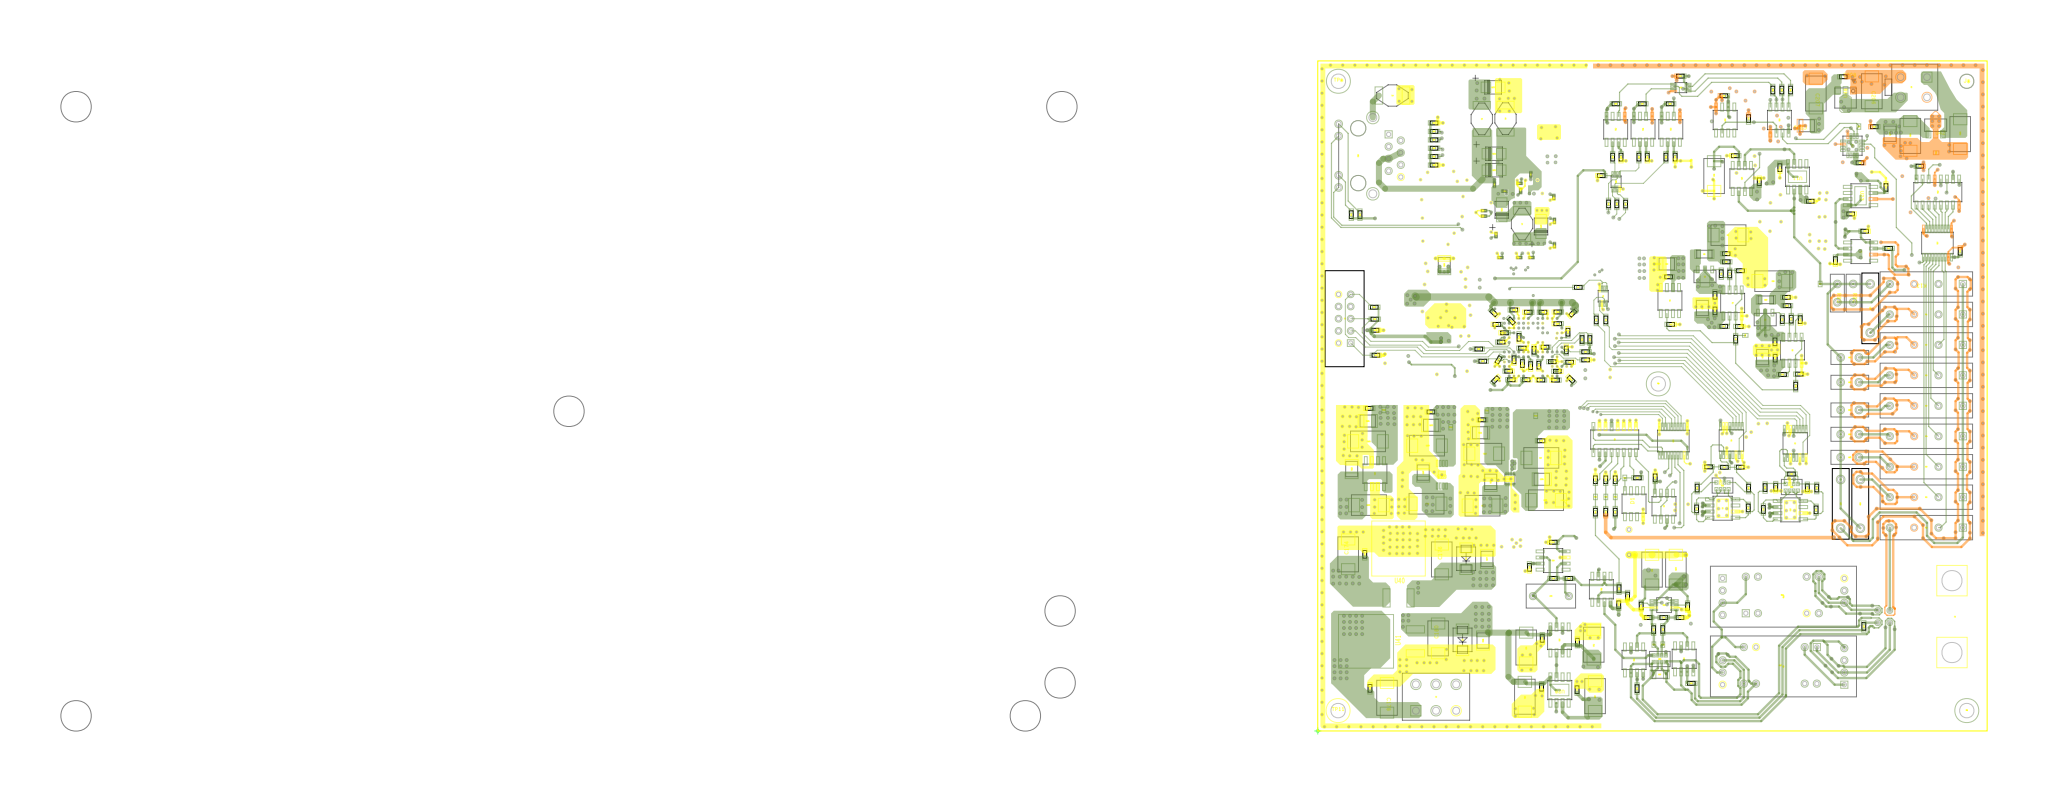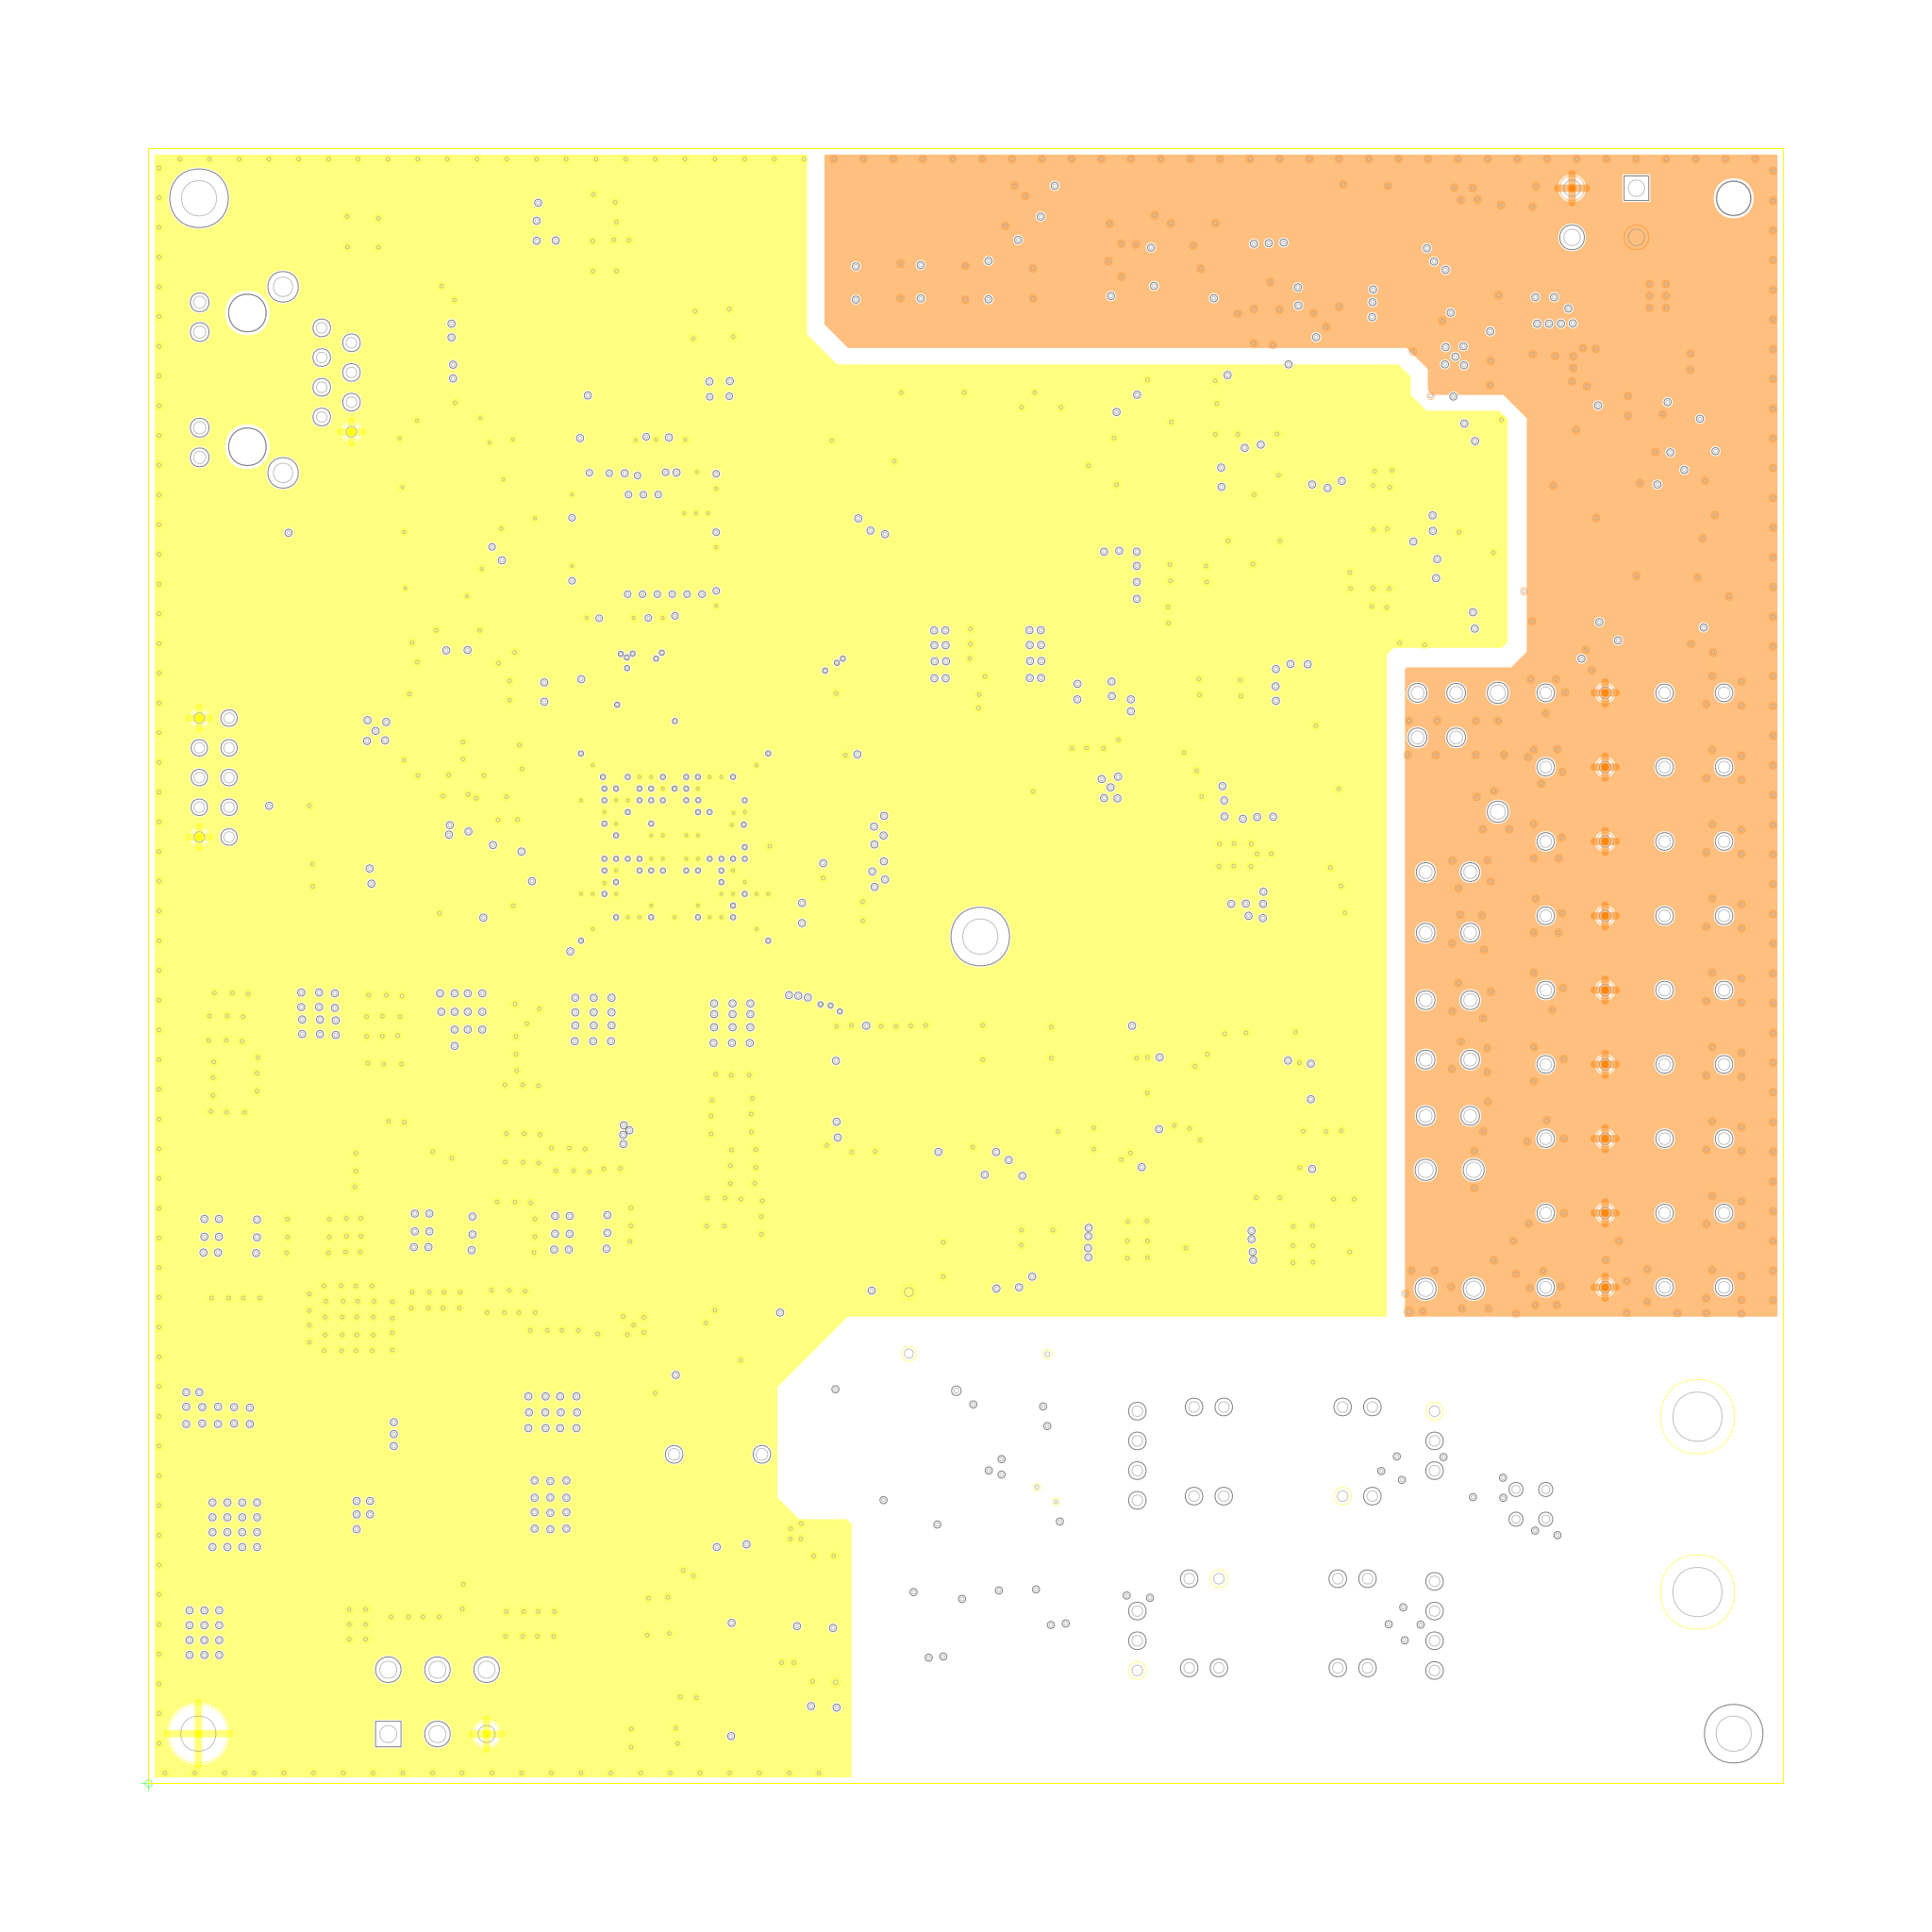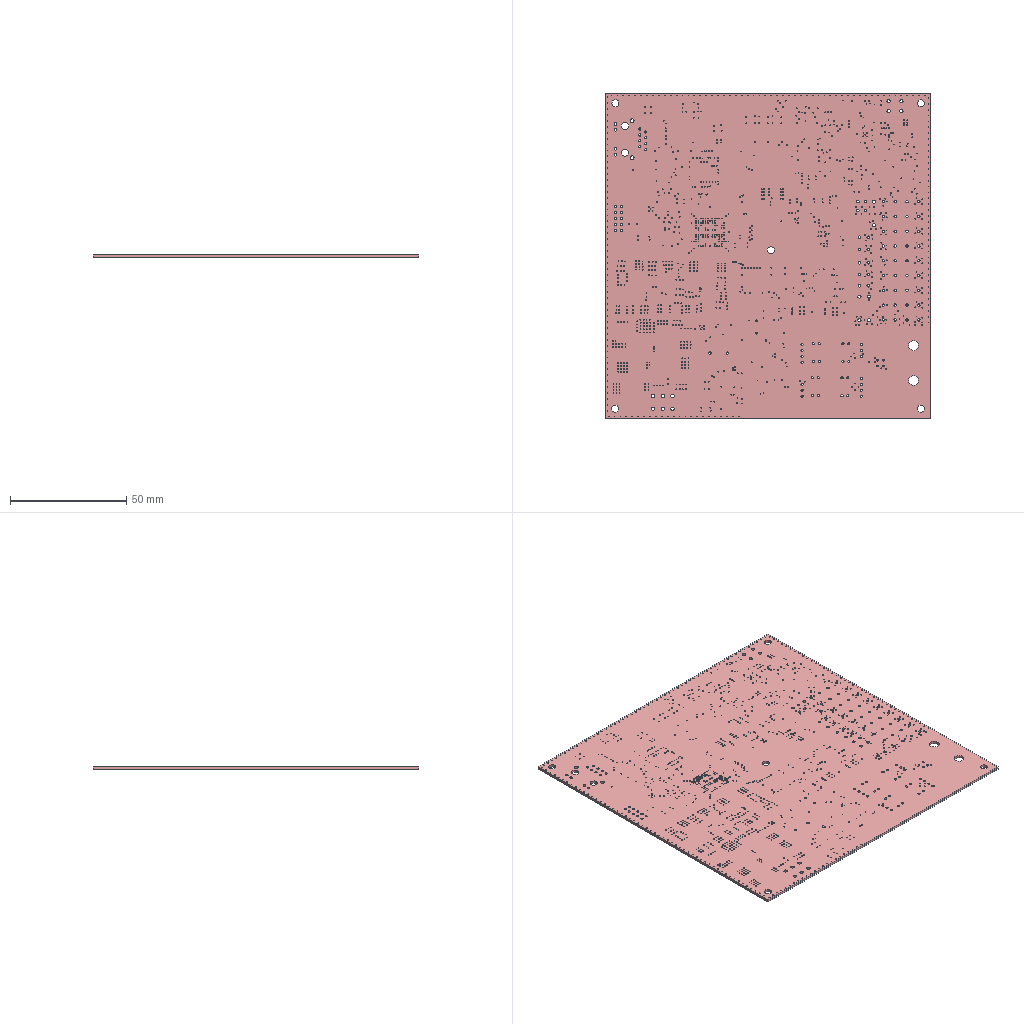Circuit board layout | Cadence Allegro | box 139.7 x 139.7 x 1.1 mm
Layer stack:
# Cadence Allegro layer stack of  (unit mm; from the constraint file cross-section; dielectric type: 0 not recorded (Allegro does not mark core vs prepreg), 3 surface material)
index,name,kind,layer,copper_thickness_mm,dielectric_type,dielectric_thickness_mm,dielectric_material,dielectric_constant
0,Top Surface,other,,,,,,
1,TOP,copper,TOP,0.0305,,,,
2,Dielectric1,dielectric,,,0,0.2032,FR-4,4.5
3,GND02,copper,GND02,0.0305,,,,
4,Dielectric2,dielectric,,,0,0.2032,FR-4,4.5
5,SIS03,copper,SIS03,0.0305,,,,
6,Dielectric3,dielectric,,,0,0.2032,FR-4,4.5
7,POW04,copper,POW04,0.0305,,,,
8,Dielectric4,dielectric,,,0,0.2032,FR-4,4.5
9,GND05,copper,GND05,0.0305,,,,
10,Dielectric5,dielectric,,,0,0.2032,FR-4,4.5
11,BOTTOM,copper,BOTTOM,0.0305,,,,
12,Bottom Surface,other,,,,,,
# drill layer pairs: low layer,high layer
drill_pair,TOP,BOTTOM
Part placement:
REFDES,COMP_VALUE,SYM_NAME,SYM_X,SYM_Y,SYM_ROTATE,SYM_MIRROR
C1,,C0603,3384.6,3751.5,270.000,NO
C2,,C0603,3263.6,3576.0,270.000,NO
C3,,C0603,3355.6,3918.0,0.000,NO
C4,,CT7343,3374.6,4070.0,0.000,NO
C5,,CT7343,3696.6,2499.0,270.000,YES
C6,,C0603,3911.6,2494.0,270.000,YES
C7,,C0603,3372.6,2403.0,0.000,YES
C8,,C0603,2882.6,3728.0,180.000,NO
C9,,C0603,3464.1,3320.0,0.000,NO
C10,,C1210,2867.6,3833.0,180.000,NO
C11,,C0603,2899.1,3337.0,0.000,NO
C12,,C1210,3160.6,3472.0,90.000,NO
C13,,C0603,3263.6,3448.0,90.000,NO
C14,,C0603,3341.6,2164.0,0.000,NO
C15,,C0603,3471.6,2165.0,0.000,NO
C16,,C0603,3210.6,2168.0,180.000,NO
C17,,C0603,3537.6,1831.0,90.000,NO
C18,,CT7343,3301.6,1695.0,180.000,YES
C19,,C0603,3039.6,1752.0,0.000,YES
C20,,C1210,3179.6,1906.0,180.000,YES
C21,,C0603,3112.6,1823.0,90.000,NO
C22,,C0603,3890.6,3380.0,270.000,NO
C23,,CT7343,3734.6,3692.0,180.000,NO
C24,,C0603,3756.6,3194.0,270.000,NO
C25,,C0603,3850.6,3559.0,0.000,NO
C26,,C0603,3561.6,2382.0,270.000,YES
C27,,CT7343,1836.6,2241.0,0.000,NO
C28,,C0603,3956.1,2929.0,0.000,NO
C29,,C1210,3654.6,3069.0,90.000,NO
C30,,C0603,3758.6,3060.0,90.000,NO
C31,,C0603,4022.6,1996.0,270.000,NO
C32,,C0603,3892.6,2109.0,0.000,NO
C33,,C0603,3762.6,2001.0,270.000,NO
C34,,C0603,2446.6,2585.0,180.000,YES
C35,,C0603,2324.6,2107.0,90.000,YES
C36,,C0603,1511.6,1447.0,270.000,YES
C37,,C0603,4094.6,1815.0,90.000,NO
C38,,CT7343,3868.6,1688.0,180.000,YES
C39,,C0603,2772.6,2078.0,90.000,NO
C40,,C0603,3604.6,1739.0,0.000,YES
C41,,C1210,3724.6,1882.0,180.000,YES
C42,,C0603,3661.6,1818.0,90.000,NO
C43,,CT7343,3256.6,4555.0,270.000,NO
C44,,C0603,4695.6,4831.0,90.000,YES
C45,,C0603,3430.6,4722.0,180.000,NO
C46,,CT7343,3966.6,4170.0,90.000,YES
C47,,C0603,4668.6,4461.0,90.000,NO
C48,,C0603,4454.6,4664.0,0.000,NO
C49,,C0603,3828.6,4902.0,0.000,YES
C50,,CT7343,3806.6,5033.0,0.000,YES
C51,,CT7343,3514.6,5126.9,270.000,YES
C52,,C0603,3539.6,5027.0,90.000,NO
C53,,C0603,3336.6,5214.0,180.000,NO
C54,,CT7343,3310.6,5125.9,270.000,YES
C55,,C0603,4322.6,4800.0,0.000,YES
C56,,C0603,4493.6,4102.0,0.000,NO
C57,,CT7343,3715.6,4302.0,270.000,YES
C58,,C0603,3627.6,4508.0,90.000,NO
C59,,CT7343,3512.6,4520.1,90.000,YES
C60,,C0603,4350.6,4698.0,90.000,YES
C61,,C0603,2462.6,4992.0,180.000,YES
C62,,C0603,4946.6,4636.0,0.000,NO
C63,,C0603,2979.6,5375.0,180.000,NO
C64,,C0603,5278.6,3937.0,90.000,NO
C65,,C0603,2672.6,4992.0,180.000,YES
C66,,CT7343,4268.6,3885.0,0.000,YES
C67,,C0603,4046.6,4348.0,0.000,NO
C68,,CT7343,4272.6,4489.0,0.000,YES
C69,,C0603,4253.6,3861.0,270.000,NO
C70,,C0603,5045.6,4330.0,0.000,YES
C71,,C0603,2903.6,4992.0,180.000,YES
C72,,CT7343,4272.6,4289.0,180.000,YES
C73,,CT7343,4273.6,4089.0,180.000,YES
C74,,C0603,3796.6,4624.0,270.000,NO
C75,,C0603,4378.6,4244.0,0.000,NO
C76,,ECQ_E1224KF,1915.6,1107.0,180.000,NO
C77,,C0603,2133.6,729.0,90.000,NO
C78,,CT7343,2267.6,707.9,90.000,NO
C79,,C0603,2130.6,339.0,90.000,NO
C80,,CT7343,2278.6,285.9,90.000,NO
C81,,C0603,1739.6,1343.0,270.000,NO
C82,,C0603,1935.6,1549.0,180.000,NO
C83,,C0603,1844.6,760.0,270.000,NO
C84,,CT7343,1712.6,684.9,90.000,NO
C85,,C0603,1838.6,359.0,270.000,NO
C86,,CT7343,1701.6,280.9,90.000,NO
C87,,C0603,2528.6,600.0,270.000,YES
C88,,C1206,2529.6,446.0,180.000,YES
C89,,C0603,2626.6,573.0,180.000,YES
C90,,C0603,2373.6,1322.0,180.000,YES
C91,,CT7343,2746.6,1324.0,90.000,NO
C92,,C0603,2714.6,931.0,0.000,NO
C93,,C0603,2657.6,1026.0,270.000,NO
C94,,C0603,2940.6,609.0,270.000,YES
C95,,C0603,2472.6,1036.0,90.000,NO
C96,,C0603,2842.6,931.0,180.000,NO
C97,,C0603,2976.6,931.0,0.000,NO
C98,,C1206,3009.6,470.0,0.000,YES
C99,,C0603,3038.6,1021.0,270.000,NO
C100,,CT7343,2942.6,1324.0,270.000,NO
C101,,C0603,3038.6,582.0,180.000,YES
C102,,C0603,2329.2,4558.5,180.000,NO
C103,,C0603,470.6,3289.0,0.000,NO
C104,,C0603,1156.6,2953.0,180.000,YES
C105,,C1210,644.6,3055.0,0.000,YES
C106,,C0603,1568.0,2953.4,0.000,NO
C107,,C0603,1485.6,3046.0,239.389,NO
C108,,C1210,1316.6,3672.0,0.000,YES
C109,,CT7343,1141.6,2322.0,90.000,YES
C110,,C0603,1534.5,3268.3,180.000,NO
C111,,C0603,1927.4,3031.3,0.000,NO
C112,,C1210,2306.6,2933.0,180.000,YES
C113,,CT7343,948.6,2318.0,90.000,YES
C114,,C0603,1610.6,3456.0,0.000,NO
C115,,C0603,1729.6,3437.0,180.000,NO
C116,,C0603,1850.6,3437.0,0.000,NO
C117,,C0603,1445.3,3432.7,315.000,NO
C118,,C0603,1972.6,3439.0,180.000,NO
C119,,C0603,2095.0,3429.2,225.000,NO
C120,,C0603,1971.6,3343.0,180.000,NO
C121,,C0603,2055.6,3273.0,90.000,NO
C122,,C0603,2081.6,2885.5,135.000,NO
C123,,C0603,1953.6,2880.0,180.000,NO
C124,,C0603,1833.6,2881.0,180.000,NO
C125,,C0603,1712.6,2883.0,0.000,NO
C126,,C0603,1589.9,2882.8,0.000,NO
C127,,C0603,1507.4,3191.9,0.000,NO
C128,,C0603,2069.4,3026.4,0.000,NO
C129,,C0603,2042.1,3127.6,90.000,NO
C130,,C0603,1145.1,3202.5,180.000,YES
C131,,C0603,1471.6,3337.0,180.000,NO
C132,,C0603,1460.0,2883.4,45.000,NO
C133,,C1210,1039.6,3824.0,90.000,NO
C134,,C0603,1103.6,3769.0,180.000,YES
C135,,C0603,970.6,3772.0,0.000,YES
C136,,C0603,1590.9,3364.8,315.000,NO
C137,,C0603,1776.6,3125.0,90.000,NO
C138,,C0603,1867.6,3150.0,180.000,NO
C139,,C0603,1748.6,2999.0,270.000,NO
C140,,C0603,1681.6,3016.0,270.000,NO
C141,,C0603,1612.6,3047.0,270.000,NO
C142,,C0603,1681.6,3142.0,0.000,NO
C143,,C0603,1968.5,2952.1,0.000,NO
C144,,C0603,1816.3,3002.6,270.000,NO
C145,,C0603,1653.6,3231.0,270.000,NO
C146,,C1210,1336.6,2585.0,0.000,YES
C147,,CT7343,1450.6,2315.0,90.000,YES
C148,,C0603,1151.6,4360.2,270.000,YES
C149,,C0603,1151.6,4242.0,90.000,YES
C150,,C0603,955.6,4991.0,180.000,NO
C151,,C3528,1448.7,4738.0,0.000,NO
C152,,C3528,1448.7,4603.0,0.000,NO
C153,,C0402,1451.6,4485.0,270.000,NO
C154,,C0603,1423.6,4639.0,270.000,YES
C155,,C3528,1834.6,4141.0,90.000,NO
C156,,C0402,1666.6,4434.0,90.000,NO
C157,,C0402,1364.6,4226.0,180.000,NO
C158,,C0402,1944.6,4186.0,270.000,NO
C159,,C0402,1754.6,3886.0,180.000,NO
C160,,C0402,1499.6,3886.0,180.000,NO
C161,,C0402,1364.6,4271.0,180.000,NO
C162,,C3528,1511.6,4278.0,90.000,NO
C163,,C0402,1750.6,4568.0,90.000,NO
C164,,C0402,1534.6,4431.0,180.000,NO
C165,,C0603,955.6,4645.0,0.000,NO
C166,,C3528,1905.6,4832.0,270.000,YES
C167,,C3528,1440.6,5283.0,0.000,NO
C168,,C0402,1656.6,4495.0,180.000,NO
C169,,C0402,1944.6,3986.0,270.000,NO
C170,,C0402,1939.6,4381.0,270.000,NO
C171,,C0402,1654.6,3886.0,180.000,NO
C172,,C0402,1464.6,4071.0,90.000,NO
C173,,C1210,4702.6,4902.0,270.000,NO
C174,,CT7343,250.0,1449.9,90.000,NO
C175,,C0603,386.0,1450.0,90.000,NO
C176,,CT7343,1019.0,1407.9,90.000,NO
C177,,C1210,1390.0,1412.0,90.000,NO
C178,,CT7343,569.0,272.1,270.000,NO
C179,,C0603,429.0,350.0,270.000,NO
C180,,CT7343,989.0,759.9,90.000,NO
C181,,C1210,1357.6,742.0,90.000,NO
C182,,CT7343,5278.6,4899.1,270.000,NO
C183,,C0603,4572.6,4960.0,180.000,NO
C184,,CT7343,4868.6,4884.1,270.000,NO
C185,,CT7343,1369.6,1507.9,270.000,YES
C186,,C0603,1882.6,1752.4,270.000,YES
C187,,CT7343,1737.6,1843.9,270.000,YES
C188,,CT7343,420.5,1854.0,0.000,NO
C189,,C1210,278.6,2150.0,90.000,NO
C190,,C0603,422.6,2648.0,180.000,NO
C191,,C1210,410.6,2544.0,180.000,NO
C192,,CT7343,412.7,2377.0,180.000,NO
C193,,C0603,1349.6,2554.0,180.000,NO
C194,,C1210,1333.6,2448.0,180.000,NO
C195,,CT7343,1367.7,2276.0,180.000,NO
C196,,CT7343,893.7,1865.0,180.000,NO
C197,,C1210,866.6,2121.0,90.000,NO
C198,,C0603,929.6,2619.0,180.000,NO
C199,,C1210,931.6,2509.0,180.000,NO
C200,,CT7343,897.7,2342.0,180.000,NO
C201,,CT7343,1353.7,1849.0,180.000,NO
C202,,C1210,1420.6,2045.0,90.000,NO
C203,,C0603,1834.6,2382.0,0.000,NO
C204,,C1210,1840.6,2066.0,0.000,NO
C205,,CT7343,1875.5,1894.0,0.000,NO
C206,,CT7343,4552.6,5251.1,270.000,NO
C207,,CT7343,4092.6,5232.1,270.000,NO
C208,,C0603,4317.6,5370.0,0.000,NO
C209,,C1210,4017.6,4968.0,180.000,NO
D1,,ASOIC_8_4MX5MX1M75_1M27,2598.7,1865.3,90.000,NO
D3,,SOT_3_1M4X3MX1M1_0M95,3838.6,689.0,180.000,YES
D5,,SOT_3_1M4X3MX1M1_0M95,3686.4,841.0,270.000,YES
D6,,SOT23,1190.1,4051.0,270.000,YES
D7,,DO-214AA,679.6,1254.0,0.000,YES
D8,,DO-214AA,1219.0,1414.0,270.000,NO
D9,,DO-214AA,1189.6,748.0,270.000,NO
D10,,DO-214AA,541.6,930.0,180.000,YES
J1,,ECG_0B_304_CLV,4650.4,938.8,180.000,NO
J2,,N2510_6002RB,220.6,3384.0,90.000,NO
J3,,39281043,5005.6,5366.7,270.000,NO
J4,,39281063,806.4,166.0,0.000,NO
K1,,COTO_9001_5_1,5000.4,3419.0,180.000,NO
K2,,COTO_9001_5_1,5000.4,1919.0,180.000,NO
K3,,COTO_9001_5_1,5000.4,2169.0,180.000,NO
K4,,COTO_9001_5_1,5000.4,2419.0,180.000,NO
K5,,COTO_9001_5_1,5000.4,2669.0,180.000,NO
K6,,COTO_9001_5_1,5000.4,2919.0,180.000,NO
K7,,COTO_9001_5_1,5000.4,3169.0,180.000,NO
K8,,COTO_9001_5_1,5000.4,1669.0,180.000,NO
K9,,COTO_3502_05_511-A,3826.4,529.8,270.000,NO
K10,,COTO_3502_05_511,3800.8,538.6,180.000,NO
K11,,COTO_3502_05_511-A,3826.4,1102.2,90.000,NO
K12,,COTO_3502_05_511,3817.1,1116.4,0.000,NO
K13,,COTO_9001_5_1,5000.4,3669.0,180.000,NO
L1,,DO1608C,1347.6,5024.0,270.000,NO
L2,,DO1608C,1678.6,4161.0,90.000,NO
L3,,DO1608C,1542.6,5026.0,270.000,NO
L4,,DO1608C,613.6,5216.0,0.000,NO
Q1,,SOT_3_2M6X4M6X1M6_1M5_C,3181.6,3788.0,180.000,NO
Q2,,SOT_3_2M6X4M6X1M6_1M5_C,3676.6,3434.0,180.000,NO
R1,,R0603,3315.6,3753.0,90.000,NO
R2,,R1206,3176.6,3914.0,0.000,NO
R3,,R0603,3356.6,3851.0,0.000,NO
R4,,R0603,3473.6,3778.0,180.000,NO
R5,,R0603,3433.6,3216.0,90.000,NO
R6,,R0603,2288.6,3374.0,90.000,NO
R7,,R0603,2140.6,3641.0,180.000,NO
R8,,R0603,3335.6,3321.0,180.000,NO
R9,,R0603,2366.6,3374.0,270.000,NO
R10,,R0603,3539.6,1994.0,90.000,NO
R11,,R0603,3117.6,1994.0,90.000,NO
R12,,R0603,3817.1,3377.0,90.000,NO
R13,,R1206,3681.6,3539.0,0.000,NO
R14,,R0603,2281.6,1796.0,90.000,NO
R15,,R0603,3855.1,3491.0,0.000,NO
R16,,R0603,2281.6,2062.0,270.000,NO
R17,,R0603,3964.6,3376.5,90.000,NO
R18,,R0603,3926.6,2831.0,90.000,NO
R19,,R0603,2365.6,1796.0,90.000,NO
R20,,R0603,2365.6,2062.0,270.000,NO
R21,,R0603,3818.6,2926.0,180.000,NO
R22,,R0603,2444.6,1796.0,90.000,NO
R23,,R0603,2444.6,2062.0,270.000,NO
R24,,R0603,4099.6,1994.0,90.000,NO
R25,,R0603,2626.6,2078.0,180.000,NO
R26,,R0603,3675.6,1998.0,90.000,NO
R27,,SM10203,4296.4,1864.0,270.000,NO
R28,,SM10203,4539.2,3469.0,270.000,NO
R29,,SM10203,4458.2,1864.0,90.000,NO
R30,,RD_2_7M87X2M91X8M53_3M81,4371.4,2246.0,0.000,NO
R31,,RD_2_7M87X2M91X8M53_3M81,4371.4,2435.0,0.000,NO
R32,,RD_2_7M87X2M91X8M53_3M81,4371.4,2635.0,0.000,NO
R33,,R0603,2449.1,5148.0,0.000,NO
R34,,R0603,2491.6,4710.0,270.000,NO
R35,,RD_2_7M87X2M91X8M53_3M81,4371.4,2862.0,0.000,NO
R36,,RD_2_7M87X2M91X8M53_3M81,4371.4,3066.0,0.000,NO
R37,,R0603,2667.1,5148.0,0.000,NO
R38,,R0603,2707.6,4710.0,270.000,NO
R39,,R0603,4690.6,3961.0,180.000,NO
R40,,R0603,2895.1,5148.0,0.000,NO
R41,,R0603,2936.6,4710.0,270.000,NO
R42,,R0603,2063.6,1252.0,0.000,NO
R43,,R0603,1936.6,1252.0,0.000,NO
R44,,R1206,2544.6,762.0,270.000,YES
R45,,R0603,2623.6,348.0,90.000,NO
R46,,R1206,2653.6,762.0,270.000,YES
R47,,R1206,2809.6,464.0,180.000,NO
R48,,R0603,2475.6,1168.0,90.000,NO
R49,,R1206,2956.6,771.0,270.000,YES
R50,,R0603,2759.6,832.0,90.000,NO
R51,,R0603,2834.6,833.0,90.000,NO
R52,,R0603,3069.6,391.0,180.000,NO
R53,,R0603,2545.6,1107.0,270.000,NO
R54,,R1206,3065.6,771.0,270.000,YES
R55,,R0603,4473.6,836.0,90.000,YES
R56,,R0603,4544.6,1110.2,0.000,YES
R57,,R0603,4486.6,858.3,270.000,NO
R58,,R0603,464.6,3478.0,0.000,NO
R59,,R0603,2171.6,3213.0,90.000,NO
R60,,R0603,1355.6,3035.0,0.000,NO
R61,,R0603,1322.6,3135.0,0.000,NO
R62,,R0603,468.6,3380.0,0.000,NO
R63,,R0603,2235.6,3213.0,90.000,NO
R64,,R0603,2200.9,3112.3,180.000,NO
R65,,R0603,477.6,3084.0,180.000,NO
R66,,R0603,2457.1,4326.4,270.000,NO
R67,,R0603,1271.6,3207.0,0.000,YES
R68,,R0603,2200.6,3046.0,0.000,NO
R69,,R0603,1148.6,3028.0,0.000,YES
R70,,R0603,2529.1,4325.0,270.000,NO
R71,,R0603,2389.1,4326.2,270.000,NO
R72,,R0603,952.6,3305.1,270.000,YES
R73,,R0603,1276.7,3295.3,0.000,YES
R74,,R0603,1223.6,4311.0,90.000,YES
R75,,R0603,1315.6,4491.0,90.000,YES
R76,,R0603,955.6,4921.0,0.000,NO
R77,,R0603,955.6,4852.0,0.000,NO
R78,,R0603,275.6,4238.0,90.000,NO
R79,,R0603,1256.6,4491.0,90.000,YES
R80,,R0603,346.6,4238.0,90.000,NO
R81,,R0603,1856.6,4627.0,90.000,YES
R82,,R0603,1921.6,4627.0,90.000,YES
R83,,R0603,1986.6,4627.0,90.000,YES
R84,,R0603,955.6,4715.0,180.000,NO
R85,,R0603,955.6,4783.0,180.000,NO
R86,,R0603,2422.6,4710.0,270.000,NO
R87,,R0603,2638.6,4710.0,270.000,NO
R88,,R0603,2860.6,4710.0,270.000,NO
R89,,R0603,3738.6,5261.0,90.000,NO
R90,,R0603,3812.6,5261.0,90.000,NO
R91,,R0603,3884.6,5261.0,90.000,NO
R92,,RD_2_7M87X2M91X8M53_3M81,4399.2,3594.0,270.000,NO
R93,,RD_2_7M87X2M91X8M53_3M81,4269.2,3594.0,270.000,NO
RN1,,ACASA,3325.6,2012.0,180.000,NO
RN2,,ACASA,3894.6,2000.0,180.000,NO
RN3,,ACASA,4275.6,4982.0,270.000,YES
RN4,,ACASA,2810.6,593.0,0.000,NO
TP1,,TP_0M8X1M15,3512.6,3247.0,270.000,NO
TP2,,TP_0M8X1M15,2281.6,1921.0,180.000,NO
TP3,,TP_0M8X1M15,2366.6,1921.0,180.000,NO
TP4,,TP_0M8X1M15,2444.6,1921.0,180.000,NO
TP5,,TP_0M8X1M15,2522.6,2077.0,180.000,NO
TP6,,TP_0M8X1M15,4445.6,4961.0,180.000,NO
TP7,,TP_0M8X1M15,4128.0,3669.0,180.000,NO
TP8,,TP_0M8X1M15,1961.6,1721.9,180.000,YES
TP9,,TP_0M8X1M15,2761.6,709.0,0.000,NO
TP10,,TP_0M8X1M15,2834.6,709.0,180.000,NO
TP11,,M3,167.2,167.2,0.000,NO
TP12,,TP_0M8X1M15,5080.6,4746.0,270.000,NO
TP13,,TP_0M8X1M15,542.6,2635.0,180.000,NO
TP14,,TP_0M8X1M15,1389.6,2630.0,180.000,NO
TP15,,TP_0M8X1M15,1092.6,2493.0,180.000,NO
TP16,,TP_0M8X1M15,1790.6,2587.0,180.000,NO
U1,,SOIC_8_4MX5MX1M75_1M27,3408.6,3513.0,90.000,NO
U2,,SOIC_8_4MX5MX1M75_1M27,2893.6,3533.0,270.000,NO
U3,,SOPTS_16_4M5X5M1X1M2_0M65,3398.6,2384.0,90.000,NO
U4,,SOPVS_8_2M4X2M1X0M9_0M5,2345.6,3569.0,270.000,NO
U5,,SOIC8,3326.6,1828.0,270.000,NO
U6,,SOIC_8_4MX5MX1M75_1M27,3900.6,3125.0,90.000,NO
U7,,SOPTS_16_4M5X5M1X1M2_0M65,3923.0,2360.9,90.000,NO
U8,,SOIC_16_4MX10MX1M75_1M27,2439.6,2392.0,90.000,NO
U9,,SOIC_8_4MX5MX1M75_1M27,2844.6,1845.0,270.000,NO
U10,,SOIC8,3883.6,1815.0,270.000,NO
U11,,TO220_5_10M67X4M83X16M11_1M7_B,3941.7,4549.0,180.000,NO
U12,,QFN_17_4MX4MX1M_0M65,4393.6,4804.0,270.000,NO
U13,,SOIC_8_4MX5MX1M75_1M27,3484.6,4535.0,90.000,NO
U14,,SOIC_8_4MX5MX1M75_1M27,4540.6,4839.0,270.000,YES
U15,,SOIC_8_4MX5MX1M75_1M27,3793.6,5015.0,270.000,NO
U16,,SOIC_8_4MX5MX1M75_1M27,3347.6,5015.0,270.000,NO
U17,,SOPTS_20_4M5X6M6X1M2_0M65,5091.6,4005.0,270.000,NO
U18,,SOIC_8_4MX5MX1M75_1M27,2447.6,4938.0,90.000,NO
U19,,SOIC_16_4MX10MX1M75_1M27,5094.6,4423.0,90.000,NO
U20,,SOPVS_8_2M4X2M1X0M9_0M5,2983.6,5281.0,0.000,NO
U21,,SOIC_8_4MX5MX1M75_1M27,2672.6,4939.0,90.000,NO
U22,,SOIC_8_4MX5MX1M75_1M27,4460.3,3935.0,180.000,NO
U23,,TO220_5_10M67X4M83X16M11_1M7_B,4459.6,4393.1,270.000,NO
U24,,SOIC_16_4MX10MX1M75_1M27,5046.6,4082.0,180.000,YES
U25,,SOIC_8_4MX5MX1M75_1M27,2900.6,4939.0,90.000,NO
U26,,SOIC_8_4MX5MX1M75_1M27,1933.6,1399.0,180.000,NO
U27,,SOIC_8_4MX5MX1M75_1M27,1986.5,747.0,270.000,NO
U28,,TO220_5_10M67X4M83X16M11_1M7_B,1988.6,336.0,180.000,NO
U29,,SOIC_8_4MX5MX1M75_1M27,2598.6,583.0,90.000,NO
U30,,SOPTS_20_4M5X6M6X1M2_0M65,2921.6,2380.0,270.000,NO
U31,,SOIC_8_4MX5MX1M75_1M27,2330.6,1163.0,90.000,NO
U32,,SOPM_10_3M1X3M1X1M1_0M5,2845.6,1033.0,180.000,NO
U33,,BGA_256_17MX17MX1M55_1M,1769.6,3150.0,180.000,YES
U34,,SOIC_8_4MX5MX1M75_1M27,924.8,3002.2,0.000,YES
U35,,SOPVS_8_2M4X2M1X0M9_0M5,1091.6,3304.1,180.000,YES
U36,,SOPVS_8_2M4X2M1X0M9_0M5,2451.3,4507.7,90.000,NO
U37,,CO4-5R0X7R0-S,1041.6,3576.0,90.000,YES
U38,,100-LQFP,1667.9,4159.4,90.000,YES
U39,,RJ45,332.4,4722.0,90.000,NO
U40,,TO-263-2,663.5,1497.5,0.000,NO
U41,,TO-263-2,396.5,735.5,90.000,NO
U42,,UA78L05ACPK_SOT_3,5077.0,4895.4,0.000,NO
U43,,SOIC_8_4MX5MX1M75_1M27,469.6,2112.0,270.000,NO
U44,,UA78L05ACPK_SOT_3,1741.2,1541.0,90.000,YES
U45,,MINI_SO_EP_8,1019.6,2103.0,180.000,NO
U46,,DFN_9_2M1X2M1X0M6_0M5,1578.6,2068.0,90.000,NO
U47,,SOIC_8_4MX5MX1M75_1M27,3010.6,592.0,90.000,NO
U48,,L79L05ABUTR,4336.4,5258.4,90.000,NO
U49,,TO220_5_10M67X4M83X16M11_1M7_B,3961.0,4630.0,180.000,YES
U50,,TO220_5_10M67X4M83X16M11_1M7_B,4703.0,4150.9,270.000,YES
U51,,TO220_5_10M67X4M83X16M11_1M7_B,2038.0,671.0,270.000,YES
Y1,,CO2-4R8X11R1-S,991.6,4299.0,270.000,YES
Pad and via stacks:
# Allegro (Cadence) via spans and padstacks; design units: ("mils" 1 10)
# via spans: padstack,start_layer,end_layer,net_example,count
VIA0M45X0M25,ETCH/TOP,ETCH/BOTTOM,GND,113
VIA10-F,ETCH/BOTTOM,ETCH/TOP,GND,48
V50D30,ETCH/TOP,ETCH/BOTTOM,GND,2
VIA10-F,ETCH/TOP,ETCH/BOTTOM,LINKLED,4
VIA24X12,ETCH/TOP,ETCH/BOTTOM,GND,1166
V32D16,ETCH/TOP,ETCH/BOTTOM,GND,4
# Allegro padstack definitions: name,start_layer,end_layer,drill,plating,holeType,type
SMD1R60X2R70,"ETCH/TOP","ETCH/TOP",0.0,"PLATED","none","smd"
SMD0R76X0R80,"ETCH/TOP","ETCH/TOP",0.0,"PLATED","none","smd"
SMD1R20X1R60,"ETCH/TOP","ETCH/TOP",0.0,"PLATED","none","smd"
SMD2R00X2R20,"ETCH/TOP","ETCH/TOP",0.0,"PLATED","none","smd"
SMD0R51X0R51,"ETCH/TOP","ETCH/TOP",0.0,"PLATED","none","smd"
SMD1R00X1R40,"ETCH/TOP","ETCH/TOP",0.0,"PLATED","none","smd"
SMD1R60X3R60,"ETCH/TOP","ETCH/TOP",0.0,"NON_PLATED","none","smd"
SMD1R00X1R00,"ETCH/TOP","ETCH/TOP",0.0,"PLATED","none","smd"
SMD65REC13,"ETCH/TOP","ETCH/TOP",0.0,"PLATED","none","smd"
SMD1R80X2R00,"ETCH/TOP","ETCH/TOP",0.0,"PLATED","none","smd"
SMDF0R28X1R80,"ETCH/TOP","ETCH/TOP",0.0,"PLATED","none","smd"
SMDF1R80X0R28,"ETCH/TOP","ETCH/TOP",0.0,"NON_PLATED","none","smd"
SMDF1R00X0R40,"ETCH/TOP","ETCH/TOP",0.0,"PLATED","none","smd"
SMD3R10X3R10,"ETCH/TOP","ETCH/TOP",0.0,"PLATED","none","smd"
SMD1R50X5R00,"ETCH/TOP","ETCH/TOP",0.0,"PLATED","none","smd"
R640_285,"ETCH/TOP","ETCH/TOP",0.0,"NON_PLATED","none","smd"
SMD1R15X0R80,"ETCH/TOP","ETCH/TOP",0.0,"PLATED","none","smd"
R1M70X0M60,"ETCH/TOP","ETCH/TOP",0.0,"PLATED","none","smd"
R198-12_55-88,"ETCH/TOP","ETCH/TOP",0.0,"NON_PLATED","none","smd"
R142-5_45,"ETCH/TOP","ETCH/TOP",0.0,"NON_PLATED","none","smd"
R294-7_175-3,"ETCH/TOP","ETCH/TOP",0.0,"NON_PLATED","none","smd"
R2M70X1M20,"ETCH/TOP","ETCH/TOP",0.0,"PLATED","none","smd"
R0M90X0M85,"ETCH/TOP","ETCH/TOP",0.0,"PLATED","none","smd"
R2M80X2M30,"ETCH/TOP","ETCH/TOP",0.0,"PLATED","none","smd"
R1M80X1M20,"ETCH/TOP","ETCH/TOP",0.0,"PLATED","none","smd"
SMD20_17,"ETCH/TOP","ETCH/TOP",0.0,"PLATED","none","smd"
R1M20X0M90,"ETCH/TOP","ETCH/TOP",0.0,"PLATED","none","smd"
R1M40X0M60,"ETCH/TOP","ETCH/TOP",0.0,"PLATED","none","smd"
SOT89_3_PIN,"ETCH/TOP","ETCH/TOP",0.0,"PLATED","none","smd"
R0M70X0M64,"ETCH/TOP","ETCH/TOP",0.0,"PLATED","none","smd"
R0M70X0M50,"ETCH/TOP","ETCH/TOP",0.0,"PLATED","none","smd"
R1M60X0M40,"ETCH/TOP","ETCH/TOP",0.0,"PLATED","none","smd"
R1M25X0M30,"ETCH/TOP","ETCH/TOP",0.0,"PLATED","none","smd"
R2M25X1M85,"ETCH/TOP","ETCH/TOP",0.0,"PLATED","none","smd"
R1M10X0M40,"ETCH/TOP","ETCH/TOP",0.0,"PLATED","none","smd"
S2M35,"ETCH/TOP","ETCH/TOP",0.0,"PLATED","none","smd"
R1M00X0M40,"ETCH/TOP","ETCH/TOP",0.0,"PLATED","none","smd"
R1M60X0M30,"ETCH/TOP","ETCH/TOP",0.0,"PLATED","none","smd"
C0M50,"ETCH/TOP","ETCH/TOP",0.0,"PLATED","none","smd"
R2M40X1M65,"ETCH/TOP","ETCH/TOP",0.0,"PLATED","none","smd"
R0M70X0M25,"ETCH/TOP","ETCH/TOP",0.0,"PLATED","none","smd"
R1M50X1M00,"ETCH/TOP","ETCH/TOP",0.0,"PLATED","none","smd"
UA78L05ACPK_PIN2,"ETCH/TOP","ETCH/TOP",0.0,"PLATED","none","smd"
R105_55,"ETCH/TOP","ETCH/TOP",0.0,"NON_PLATED","none","smd"
R1M70X1M10,"ETCH/TOP","ETCH/TOP",0.0,"PLATED","none","smd"
R0M60X0M25,"ETCH/TOP","ETCH/TOP",0.0,"PLATED","none","smd"
R1M70X0M80,"ETCH/TOP","ETCH/TOP",0.0,"PLATED","none","smd"
THC2R60D1R65,"ETCH/TOP","ETCH/BOTTOM",65.0,"PLATED","circle_drill","through"
THC1R60D1R05,"ETCH/TOP","ETCH/BOTTOM",41.3,"PLATED","circle_drill","through"
THC0R00D3R20,"ETCH/TOP","ETCH/BOTTOM",126.0,"NON_PLATED","circle_drill","through"
THC1R50D0R90,"ETCH/TOP","ETCH/BOTTOM",35.4,"PLATED","circle_drill","through"
THS1R50D0R90,"ETCH/TOP","ETCH/BOTTOM",35.4,"PLATED","circle_drill","through"
CD1M30X0M90,"ETCH/TOP","ETCH/BOTTOM",35.4,"PLATED","circle_drill","through"
CD1M50X1M00,"ETCH/TOP","ETCH/BOTTOM",39.4,"PLATED","circle_drill","through"
CD50X28,"ETCH/TOP","ETCH/BOTTOM",28.7,"PLATED","circle_drill","through"
C123_H73,"ETCH/TOP","ETCH/BOTTOM",28.7,"PLATED","circle_drill","through"
CD1M40X0M90,"ETCH/TOP","ETCH/BOTTOM",35.4,"PLATED","circle_drill","through"
SD1M40X0M90,"ETCH/TOP","ETCH/BOTTOM",35.4,"PLATED","circle_drill","through"
CD1M20X0M70,"ETCH/TOP","ETCH/BOTTOM",27.6,"PLATED","circle_drill","through"
SD6M35X4M20,"ETCH/TOP","ETCH/BOTTOM",165.4,"PLATED","circle_drill","through"
S217-5_H145,"ETCH/TOP","ETCH/BOTTOM",57.1,"PLATED","circle_drill","through"
C217-5_H145,"ETCH/TOP","ETCH/BOTTOM",57.1,"PLATED","circle_drill","through"
SD1M50X1M00,"ETCH/TOP","ETCH/BOTTOM",39.4,"PLATED","circle_drill","through"
CD1M50X0M90,"ETCH/TOP","ETCH/BOTTOM",35.4,"PLATED","circle_drill","through"
SD1M50X0M90,"ETCH/TOP","ETCH/BOTTOM",35.4,"PLATED","circle_drill","through"
CD1M80X1M30,"ETCH/TOP","ETCH/BOTTOM",51.2,"PLATED","circle_drill","through"
CD1M60X1M10,"ETCH/TOP","ETCH/BOTTOM",43.3,"PLATED","circle_drill","through"
SD6M35X4M20_NP,"ETCH/TOP","ETCH/BOTTOM",165.4,"NON_PLATED","circle_drill","through"
SD1M80X1M30,"ETCH/TOP","ETCH/BOTTOM",51.2,"PLATED","circle_drill","through"
S210_H140,"ETCH/TOP","ETCH/BOTTOM",55.1,"PLATED","circle_drill","through"
C210_H140,"ETCH/TOP","ETCH/BOTTOM",55.1,"PLATED","circle_drill","through"
VIA24X12,"ETCH/TOP","ETCH/BOTTOM",12.0,"PLATED","circle_drill","through"
VIA0M45X0M25,"ETCH/TOP","ETCH/BOTTOM",9.8,"PLATED","circle_drill","through"
VIA,"ETCH/TOP","ETCH/BOTTOM",13.0,"PLATED","circle_drill","through"
VIA10-F,"ETCH/TOP","ETCH/BOTTOM",9.8,"PLATED","circle_drill","through"
VIA24X12_S,"ETCH/TOP","ETCH/BOTTOM",12.0,"PLATED","circle_drill","through"
R0M90X0M85-1,"ETCH/TOP","ETCH/TOP",0.0,"PLATED","none","smd"
PAD156,"ETCH/TOP","ETCH/BOTTOM",156.0,"NON_PLATED","circle_drill","through"
HOLE109P,"ETCH/TOP","ETCH/BOTTOM",108.0,"PLATED","circle_drill","through"
PAD125,"ETCH/TOP","ETCH/BOTTOM",126.0,"NON_PLATED","circle_drill","through"
SMD2M61_2M02,"ETCH/TOP","ETCH/TOP",0.0,"PLATED","none","smd"
SMD71_25,"ETCH/TOP","ETCH/TOP",0.0,"PLATED","none","smd"
SMD3M80_2M40,"ETCH/TOP","ETCH/TOP",0.0,"PLATED","none","smd"
A_SOT89,"ETCH/TOP","ETCH/TOP",0.0,"NON_PLATED","none","smd"
R45X60,"ETCH/TOP","ETCH/TOP",0.0,"NON_PLATED","none","smd"
SMD3M00_1M60,"ETCH/TOP","ETCH/TOP",0.0,"PLATED","none","smd"
SMD6M20_5M80,"ETCH/TOP","ETCH/TOP",0.0,"PLATED","none","smd"
SMD0M35_1M30,"ETCH/TOP","ETCH/TOP",0.0,"PLATED","none","smd"
PAD5M00CIR2M03D,"ETCH/TOP","ETCH/BOTTOM",118.1,"PLATED","circle_drill","through"
V32D16,"ETCH/TOP","ETCH/BOTTOM",16.0,"PLATED","circle_drill","through"
V50D30,"ETCH/TOP","ETCH/BOTTOM",30.0,"PLATED","circle_drill","through"
R1_52X3_81,"ETCH/TOP","ETCH/TOP",0.0,"PLATED","none","smd"
R11_18X11_48-NSP,"ETCH/TOP","ETCH/TOP",0.0,"PLATED","none","smd"
R1_5X1_6,"ETCH/TOP","ETCH/TOP",0.0,"NON_PLATED","none","smd"
HOLE1P9,"ETCH/TOP","ETCH/BOTTOM",74.8,"NON_PLATED","circle_drill","through"
H0300,"ETCH/TOP","ETCH/BOTTOM",118.1,"NON_PLATED","circle_drill","through"
Design rules, without the lines most boards share, first 11 of 48 lines:
# Cadence Allegro design rules of  (from the Constraint Manager export constraints.dcfx, design unit mil; typed fields in mm)
# columns: name | kind | enabled | priority | scope1 | scope2 | descriptor | typed fields (field=value)
# Allegro precedence (priority 1 wins): 1 Region class-to-class, 2 Region class, 3 Region, 4 class-to-class, 5 DiffPair/Bus/NetGroup override, 6 NetClass, 7 constraint set (CSet) default
# per-layer values are written LAYER=value in the descriptor and LAYER:mm in the typed field; a maximum of 0 means no limit set
# --- net classes (and buses / net groups) ---
# (no net classes defined: every net uses the default constraint sets)
# --- track widths, neck and differential-pair gap (physical constraint sets) ---
DEFAULT | PhysicalCSet | enabled | 7 | Design default | All | Physical Constraint (Min Line Width=6mil) (Max Line Width=0mil) (Min Neck Width=6mil) (Max Neck Length=0mil) (DiffPair Primary Gap=0mil) (DiffPair Neck Gap=0mil) (DiffPair Min Space=0mil) (DiffPair Coupled +Tol=0mil) (DiffPair Coupled -Tol=0mil) (Min BB Via Stagger=5mil) (Max BB Via Stagger=0mil) (T-junctions=ANYWHERE) (Pad-pad direct connect=ALL_ALLOWED) (Allowed vias=VIA24X12, VIA0M45X0M25, VIA10-F) | min_line_width=0.1524 min_neck_width=0.1524 min_bvia_stagger=0.127 max_bvia_stagger=0 ts_allowed=ANYWHERE diffp_primary_gap=0 diffp_neck_gap=0 max_line_width=0 maximum_neck_length=0 pad_pad_direct_connect=ALL_ALLOWED allow_on_etch_subclass=TRUE diffp_coupled_plus=0 diffp_coupled_minus=0 diffp_min_space=0 vias=VIA24X12,VIA0M45X0M25,VIA10-F
# --- clearances: line / pad / via / shape / hole (spacing constraint sets) ---
HAP | SpacingCSet | enabled | 7 | Region(1): 10 | All | Clearance Constraint (Line-Line=8mil) (Line-SMD Pad=6mil) (Line-Thru Pin=6mil) (Line-Via=7mil) (Line-Shape=TOP=10mil GND02=10mil SIS03=10mil POW04=20mil GND05=20mil BOTTOM=10mil) (SMD Pad-SMD Pad=5mil) (Thru Pin-Thru Pin=5mil) (Thru Pin-SMD Pad=5mil) (SMD Pad-Via=5mil) (Thru Pin-Via=5mil) (Via-Via=5mil) (Shape-SMD Pad=5mil) (Shape-Thru Pin=5mil) (Shape-Via=5mil) (Shape-Shape=TOP=10mil GND02=40mil SIS03=20mil POW04=20mil GND05=20mil BOTTOM=10mil) (Hole-Hole=8mil) (Hole-Line=8mil) (Hole-Shape=8mil) (BB Via-BB Via=5mil) (uVia-uVia=5mil) | thrupin_to_thrupin_spacing=0.127 thrupin_to_smdpin_spacing=0.127 thrupin_to_thruvia_spacing=0.127 line_to_thrupin_spacing=0.1524 thrupin_to_shape_spacing=0.127 smdpin_to_smdpin_spacing=0.127 smdpin_to_thruvia_spacing=0.127 line_to_smdpin_spacing=0.1524 shape_to_smdpin_spacing=0.127 thruvia_to_thruvia_spacing=0.127 line_to_thruvia_spacing=0.1778 shape_to_thruvia_spacing=0.127 line_to_line_spacing=0.2032 line_to_shape_spacing=TOP:0.254,GND02:0.254,SIS03:0.254,POW04:0.508,GND05:0.508,BOTTOM:0.254 shape_to_shape_spacing=TOP:0.254,GND02:1.016,SIS03:0.508,POW04:0.508,GND05:0.508,BOTTOM:0.254 bbv_to_bbv_spacing=0.127 bbv_to_thrupin_spacing=0.127 bbv_to_smdpin_spacing=0.127 bbv_to_thruvia_spacing=0.127 bbv_to_line_spacing=0.1778 bbv_to_shape_spacing=0.127 bbv_to_testpin_spacing=0.127 bbv_to_testvia_spacing=0.127 testpin_to_testpin_spacing=0.127 testpin_to_thrupin_spacing=0.127 smdpin_to_testpin_spacing=0.127 testpin_to_thruvia_spacing=0.127 testpin_to_testvia_spacing=0.127 line_to_testpin_spacing=0.1524 shape_to_testpin_spacing=0.127 testvia_to_testvia_spacing=0.127 testvia_to_thrupin_spacing=0.127 smdpin_to_testvia_spacing=0.127 testvia_to_thruvia_spacing=0.127 line_to_testvia_spacing=0.1778 shape_to_testvia_spacing=0.127 bondpad_to_bondpad_spacing=0.127 thrupin_to_bondpad_spacing=0.127 smdpin_to_bondpad_spacing=0.127 bondpad_to_thruvia_spacing=0.127 bondpad_to_line_spacing=0.1778 bondpad_to_shape_spacing=0.127 bondpad_to_bbv_spacing=0.127 bondpad_to_testpin_spacing=0.127 bondpad_to_testvia_spacing=0.127 min_bvia_gap=0.127 hole_to_pin_spacing=0.2032 hole_to_via_spacing=0.2032 hole_to_line_spacing=0.2032 hole_to_shape_spacing=0.2032 hole_to_hole_spacing=0.2032 mvia_to_mvia_spacing=0.127 mvia_to_thrupin_spacing=0.127 mvia_to_smdpin_spacing=0.127 mvia_to_thruvia_spacing=0.127 mvia_to_bbv_spacing=0.127 mvia_to_line_spacing=0.127 mvia_to_shape_spacing=0.127 mvia_to_testpin_spacing=0.127 mvia_to_testvia_spacing=0.127 bondpad_to_mvia_spacing=0.127 bondpad_to_bondpad_diffp_spc=0.127
DEFAULT | SpacingCSet | enabled | 7 | Design default | All | Clearance Constraint (Line-Line=8mil) (Line-SMD Pad=6mil) (Line-Thru Pin=6mil) (Line-Via=7mil) (Line-Shape=TOP=10mil GND02=10mil SIS03=10mil POW04=20mil GND05=20mil BOTTOM=10mil) (SMD Pad-SMD Pad=5mil) (Thru Pin-Thru Pin=5mil) (Thru Pin-SMD Pad=5mil) (SMD Pad-Via=5mil) (Thru Pin-Via=5mil) (Via-Via=5mil) (Shape-SMD Pad=5mil) (Shape-Thru Pin=5mil) (Shape-Via=5mil) (Shape-Shape=TOP=20mil GND02=40mil SIS03=20mil POW04=20mil GND05=20mil BOTTOM=20mil) (Hole-Hole=8mil) (Hole-Line=8mil) (Hole-Shape=8mil) (BB Via-BB Via=5mil) (uVia-uVia=5mil) | thrupin_to_thrupin_spacing=0.127 thrupin_to_smdpin_spacing=0.127 thrupin_to_thruvia_spacing=0.127 line_to_thrupin_spacing=0.1524 thrupin_to_shape_spacing=0.127 smdpin_to_smdpin_spacing=0.127 smdpin_to_thruvia_spacing=0.127 line_to_smdpin_spacing=0.1524 shape_to_smdpin_spacing=0.127 thruvia_to_thruvia_spacing=0.127 line_to_thruvia_spacing=0.1778 shape_to_thruvia_spacing=0.127 line_to_line_spacing=0.2032 line_to_shape_spacing=TOP:0.254,GND02:0.254,SIS03:0.254,POW04:0.508,GND05:0.508,BOTTOM:0.254 shape_to_shape_spacing=TOP:0.508,GND02:1.016,SIS03:0.508,POW04:0.508,GND05:0.508,BOTTOM:0.508 bbv_to_bbv_spacing=0.127 bbv_to_thrupin_spacing=0.127 bbv_to_smdpin_spacing=0.127 bbv_to_thruvia_spacing=0.127 bbv_to_line_spacing=0.1778 bbv_to_shape_spacing=0.127 bbv_to_testpin_spacing=0.127 bbv_to_testvia_spacing=0.127 testpin_to_testpin_spacing=0.127 testpin_to_thrupin_spacing=0.127 smdpin_to_testpin_spacing=0.127 testpin_to_thruvia_spacing=0.127 testpin_to_testvia_spacing=0.127 line_to_testpin_spacing=0.1524 shape_to_testpin_spacing=0.127 testvia_to_testvia_spacing=0.127 testvia_to_thrupin_spacing=0.127 smdpin_to_testvia_spacing=0.127 testvia_to_thruvia_spacing=0.127 line_to_testvia_spacing=0.1778 shape_to_testvia_spacing=0.127 bondpad_to_bondpad_spacing=0.127 thrupin_to_bondpad_spacing=0.127 smdpin_to_bondpad_spacing=0.127 bondpad_to_thruvia_spacing=0.127 bondpad_to_line_spacing=0.1778 bondpad_to_shape_spacing=0.127 bondpad_to_bbv_spacing=0.127 bondpad_to_testpin_spacing=0.127 bondpad_to_testvia_spacing=0.127 min_bvia_gap=0.127 hole_to_pin_spacing=0.2032 hole_to_via_spacing=0.2032 hole_to_line_spacing=0.2032 hole_to_shape_spacing=0.2032 hole_to_hole_spacing=0.2032 mvia_to_mvia_spacing=0.127 mvia_to_thrupin_spacing=0.127 mvia_to_smdpin_spacing=0.127 mvia_to_thruvia_spacing=0.127 mvia_to_bbv_spacing=0.127 mvia_to_line_spacing=0.127 mvia_to_shape_spacing=0.127 mvia_to_testpin_spacing=0.127 mvia_to_testvia_spacing=0.127 bondpad_to_mvia_spacing=0.127 bondpad_to_bondpad_diffp_spc=0.127